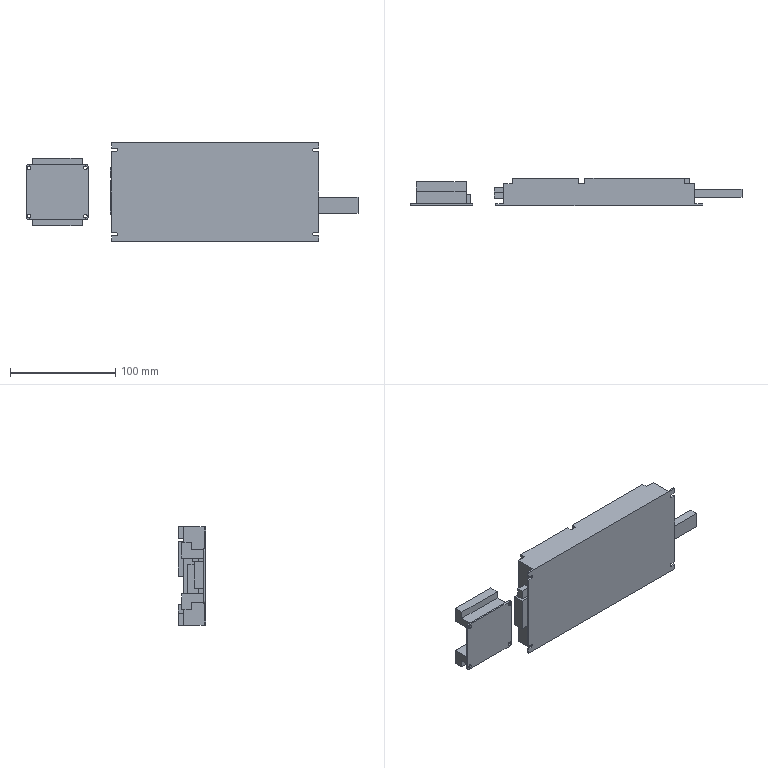Part | STEP file | 2 solids | 402 faces | box 316 x 26 x 94 mm | volume 418687 mm3 | plane 290 | spline 94 | cylinder 18 | commonest cylinder face diameters 3.5 x8 3.3 x6 5 x4